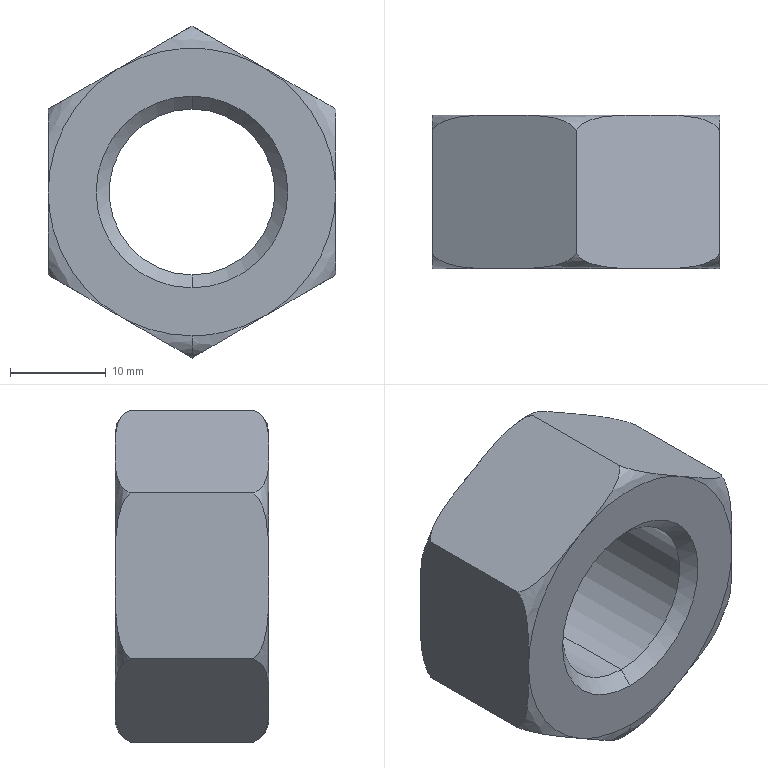Part | SolidWorks | features BaseBody 1 | 1 solid | 28 faces | box 30 x 16 x 34.641 mm | volume 8584 mm3 | spline 14 | plane 8 | cone 4 | cylinder 2 | commonest cylinder face diameters 17.294 x2